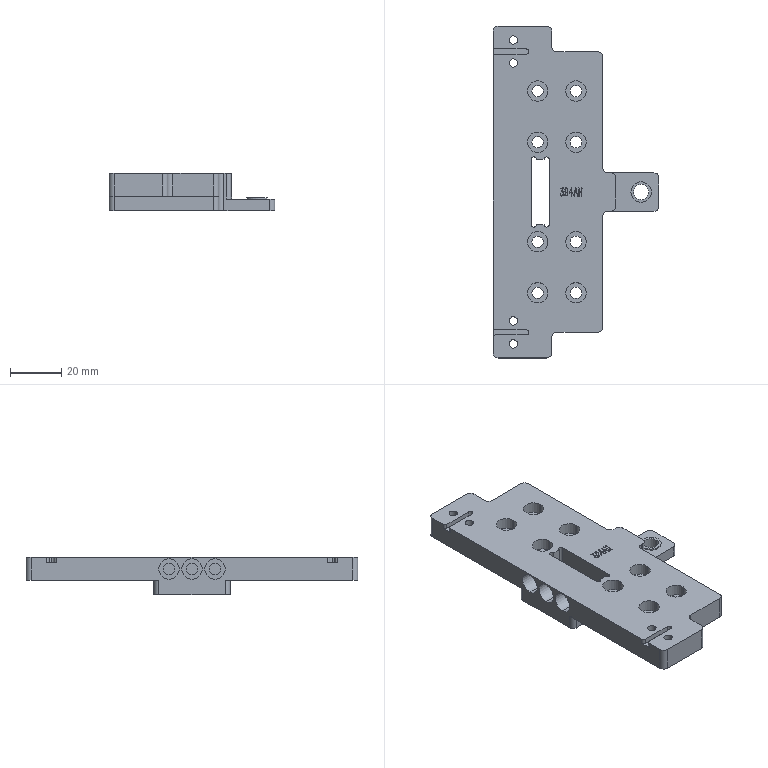NC program | NX | posted with a generic post | part box 65 x 130 x 14.5 mm
Lines 4087 to 4982 of 11202:
(ZLEVEL_PROFILE_COPY_COPY , TOOL : D3)
N8088 T16 M6
N8090 G54
N8092 G17 G0 G90 X9.873 Y-15.4 B0. C0. S9500 M3
N8094 G43 Z30. H16
N8096 Z-0.199
N8098 G94 G1 X10.133 Y-15.85 F1000.
N8100 G3 X10.393 Y-16. R0.3
N8102 G1 X11.336 F1200.
N8104 G2 X11.25 Y-15.5 R1.5
N8106 G1 Y-15.124
N8108 G3 X11.1 Y-14.864 R0.3
N8110 G1 X10.65 Y-14.604
N8112 G0 X9.873 Y-15.4 Z-0.397
N8114 G1 X10.133 Y-15.85 F1000.
N8116 G3 X10.393 Y-16. R0.3
N8118 G1 X11.336 F1200.
N8120 G2 X11.25 Y-15.5 R1.5
N8122 G1 Y-15.124
N8124 G3 X11.1 Y-14.864 R0.3
N8126 G1 X10.65 Y-14.604
N8128 G0 X9.873 Y-15.4 Z-0.596
N8130 G1 X10.133 Y-15.85 F1000.
N8132 G3 X10.393 Y-16. R0.3
N8134 G1 X11.336 F1200.
N8136 G2 X11.25 Y-15.5 R1.5
N8138 G1 Y-15.124
N8140 G3 X11.1 Y-14.864 R0.3
N8142 G1 X10.65 Y-14.604
N8144 G0 X9.873 Y-15.4 Z-0.795
N8146 G1 X10.133 Y-15.85 F1000.
N8148 G3 X10.393 Y-16. R0.3
N8150 G1 X11.336 F1200.
N8152 G2 X11.25 Y-15.5 R1.5
N8154 G1 Y-15.124
N8156 G3 X11.1 Y-14.864 R0.3
N8158 G1 X10.65 Y-14.604
N8160 G0 X9.873 Y-15.4 Z-0.993
N8162 G1 X10.133 Y-15.85 F1000.
N8164 G3 X10.393 Y-16. R0.3
N8166 G1 X11.336 F1200.
N8168 G2 X11.25 Y-15.5 R1.5
N8170 G1 Y-15.124
N8172 G3 X11.1 Y-14.864 R0.3
N8174 G1 X10.65 Y-14.604
N8176 G0 X9.873 Y-15.4 Z-1.192
N8178 G1 X10.133 Y-15.85 F1000.
N8180 G3 X10.393 Y-16. R0.3
N8182 G1 X11.336 F1200.
N8184 G2 X11.25 Y-15.5 R1.5
N8186 G1 Y-15.124
N8188 G3 X11.1 Y-14.864 R0.3
N8190 G1 X10.65 Y-14.604
N8192 G0 X9.873 Y-15.4 Z-1.39
N8194 G1 X10.133 Y-15.85 F1000.
N8196 G3 X10.393 Y-16. R0.3
N8198 G1 X11.336 F1200.
N8200 G2 X11.25 Y-15.5 R1.5
N8202 G1 Y-15.124
N8204 G3 X11.1 Y-14.864 R0.3
N8206 G1 X10.65 Y-14.604
N8208 G0 X9.873 Y-15.4 Z-1.589
N8210 G1 X10.133 Y-15.85 F1000.
N8212 G3 X10.393 Y-16. R0.3
N8214 G1 X11.336 F1200.
N8216 G2 X11.25 Y-15.5 R1.5
N8218 G1 Y-15.124
N8220 G3 X11.1 Y-14.864 R0.3
N8222 G1 X10.65 Y-14.604
N8224 G0 X9.873 Y-15.4 Z-1.788
N8226 G1 X10.133 Y-15.85 F1000.
N8228 G3 X10.393 Y-16. R0.3
N8230 G1 X11.336 F1200.
N8232 G2 X11.25 Y-15.5 R1.5
N8234 G1 Y-15.124
N8236 G3 X11.1 Y-14.864 R0.3
N8238 G1 X10.65 Y-14.604
N8240 G0 X9.873 Y-15.4 Z-1.986
N8242 G1 X10.133 Y-15.85 F1000.
N8244 G3 X10.393 Y-16. R0.3
N8246 G1 X11.336 F1200.
N8248 G2 X11.25 Y-15.5 R1.5
N8250 G1 Y-15.124
N8252 G3 X11.1 Y-14.864 R0.3
N8254 G1 X10.65 Y-14.604
N8256 G0 X9.873 Y-15.4 Z-2.185
N8258 G1 X10.133 Y-15.85 F1000.
N8260 G3 X10.393 Y-16. R0.3
N8262 G1 X11.336 F1200.
N8264 G2 X11.25 Y-15.5 R1.5
N8266 G1 Y-15.124
N8268 G3 X11.1 Y-14.864 R0.3
N8270 G1 X10.65 Y-14.604
N8272 G0 X9.873 Y-15.4 Z-2.384
N8274 G1 X10.133 Y-15.85 F1000.
N8276 G3 X10.393 Y-16. R0.3
N8278 G1 X11.336 F1200.
N8280 G2 X11.25 Y-15.5 R1.5
N8282 G1 Y-15.124
N8284 G3 X11.1 Y-14.864 R0.3
N8286 G1 X10.65 Y-14.604
N8288 G0 X9.873 Y-15.4 Z-2.582
N8290 G1 X10.133 Y-15.85 F1000.
N8292 G3 X10.393 Y-16. R0.3
N8294 G1 X11.336 F1200.
N8296 G2 X11.25 Y-15.5 R1.5
N8298 G1 Y-15.124
N8300 G3 X11.1 Y-14.864 R0.3
N8302 G1 X10.65 Y-14.604
N8304 G0 X9.873 Y-15.4 Z-2.781
N8306 G1 X10.133 Y-15.85 F1000.
N8308 G3 X10.393 Y-16. R0.3
N8310 G1 X11.336 F1200.
N8312 G2 X11.25 Y-15.5 R1.5
N8314 G1 Y-15.124
N8316 G3 X11.1 Y-14.864 R0.3
N8318 G1 X10.65 Y-14.604
N8320 G0 X9.873 Y-15.4 Z-2.979
N8322 G1 X10.133 Y-15.85 F1000.
N8324 G3 X10.393 Y-16. R0.3
N8326 G1 X11.336 F1200.
N8328 G2 X11.25 Y-15.5 R1.5
N8330 G1 Y-15.124
N8332 G3 X11.1 Y-14.864 R0.3
N8334 G1 X10.65 Y-14.604
N8336 G0 X9.873 Y-15.4 Z-3.178
N8338 G1 X10.133 Y-15.85 F1000.
N8340 G3 X10.393 Y-16. R0.3
N8342 G1 X11.336 F1200.
N8344 G2 X11.25 Y-15.5 R1.5
N8346 G1 Y-15.124
N8348 G3 X11.1 Y-14.864 R0.3
N8350 G1 X10.65 Y-14.604
N8352 G0 X9.873 Y-15.4 Z-3.377
N8354 G1 X10.133 Y-15.85 F1000.
N8356 G3 X10.393 Y-16. R0.3
N8358 G1 X11.336 F1200.
N8360 G2 X11.25 Y-15.5 R1.5
N8362 G1 Y-15.124
N8364 G3 X11.1 Y-14.864 R0.3
N8366 G1 X10.65 Y-14.604
N8368 G0 X9.873 Y-15.4 Z-3.575
N8370 G1 X10.133 Y-15.85 F1000.
N8372 G3 X10.393 Y-16. R0.3
N8374 G1 X11.336 F1200.
N8376 G2 X11.25 Y-15.5 R1.5
N8378 G1 Y-15.124
N8380 G3 X11.1 Y-14.864 R0.3
N8382 G1 X10.65 Y-14.604
N8384 G0 X9.873 Y-15.4 Z-3.774
N8386 G1 X10.133 Y-15.85 F1000.
N8388 G3 X10.393 Y-16. R0.3
N8390 G1 X11.336 F1200.
N8392 G2 X11.25 Y-15.5 R1.5
N8394 G1 Y-15.124
N8396 G3 X11.1 Y-14.864 R0.3
N8398 G1 X10.65 Y-14.604
N8400 G0 X9.873 Y-15.4 Z-3.973
N8402 G1 X10.133 Y-15.85 F1000.
N8404 G3 X10.393 Y-16. R0.3
N8406 G1 X11.336 F1200.
N8408 G2 X11.25 Y-15.5 R1.5
N8410 G1 Y-15.124
N8412 G3 X11.1 Y-14.864 R0.3
N8414 G1 X10.65 Y-14.604
N8416 G0 X9.873 Y-15.4 Z-4.171
N8418 G1 X10.133 Y-15.85 F1000.
N8420 G3 X10.393 Y-16. R0.3
N8422 G1 X11.336 F1200.
N8424 G2 X11.25 Y-15.5 R1.5
N8426 G1 Y-15.124
N8428 G3 X11.1 Y-14.864 R0.3
N8430 G1 X10.65 Y-14.604
N8432 G0 X9.873 Y-15.4 Z-4.37
N8434 G1 X10.133 Y-15.85 F1000.
N8436 G3 X10.393 Y-16. R0.3
N8438 G1 X11.336 F1200.
N8440 G2 X11.25 Y-15.5 R1.5
N8442 G1 Y-15.124
N8444 G3 X11.1 Y-14.864 R0.3
N8446 G1 X10.65 Y-14.604
N8448 G0 X9.873 Y-15.4 Z-4.568
N8450 G1 X10.133 Y-15.85 F1000.
N8452 G3 X10.393 Y-16. R0.3
N8454 G1 X11.336 F1200.
N8456 G2 X11.25 Y-15.5 R1.5
N8458 G1 Y-15.124
N8460 G3 X11.1 Y-14.864 R0.3
N8462 G1 X10.65 Y-14.604
N8464 G0 X9.873 Y-15.4 Z-4.767
N8466 G1 X10.133 Y-15.85 F1000.
N8468 G3 X10.393 Y-16. R0.3
N8470 G1 X11.336 F1200.
N8472 G2 X11.25 Y-15.5 R1.5
N8474 G1 Y-15.124
N8476 G3 X11.1 Y-14.864 R0.3
N8478 G1 X10.65 Y-14.604
N8480 G0 X9.873 Y-15.4 Z-4.966
N8482 G1 X10.133 Y-15.85 F1000.
N8484 G3 X10.393 Y-16. R0.3
N8486 G1 X11.336 F1200.
N8488 G2 X11.25 Y-15.5 R1.5
N8490 G1 Y-15.124
N8492 G3 X11.1 Y-14.864 R0.3
N8494 G1 X10.65 Y-14.604
N8496 G0 X9.873 Y-15.4 Z-5.164
N8498 G1 X10.133 Y-15.85 F1000.
N8500 G3 X10.393 Y-16. R0.3
N8502 G1 X11.336 F1200.
N8504 G2 X11.25 Y-15.5 R1.5
N8506 G1 Y-15.124
N8508 G3 X11.1 Y-14.864 R0.3
N8510 G1 X10.65 Y-14.604
N8512 G0 X9.873 Y-15.4 Z-5.363
N8514 G1 X10.133 Y-15.85 F1000.
N8516 G3 X10.393 Y-16. R0.3
N8518 G1 X11.336 F1200.
N8520 G2 X11.25 Y-15.5 R1.5
N8522 G1 Y-15.124
N8524 G3 X11.1 Y-14.864 R0.3
N8526 G1 X10.65 Y-14.604
N8528 G0 X9.873 Y-15.4 Z-5.562
N8530 G1 X10.133 Y-15.85 F1000.
N8532 G3 X10.393 Y-16. R0.3
N8534 G1 X11.336 F1200.
N8536 G2 X11.25 Y-15.5 R1.5
N8538 G1 Y-15.124
N8540 G3 X11.1 Y-14.864 R0.3
N8542 G1 X10.65 Y-14.604
N8544 G0 X9.873 Y-15.4 Z-5.76
N8546 G1 X10.133 Y-15.85 F1000.
N8548 G3 X10.393 Y-16. R0.3
N8550 G1 X11.336 F1200.
N8552 G2 X11.25 Y-15.5 R1.5
N8554 G1 Y-15.124
N8556 G3 X11.1 Y-14.864 R0.3
N8558 G1 X10.65 Y-14.604
N8560 G0 X9.873 Y-15.4 Z-5.959
N8562 G1 X10.133 Y-15.85 F1000.
N8564 G3 X10.393 Y-16. R0.3
N8566 G1 X11.336 F1200.
N8568 G2 X11.25 Y-15.5 R1.5
N8570 G1 Y-15.124
N8572 G3 X11.1 Y-14.864 R0.3
N8574 G1 X10.65 Y-14.604
N8576 G0 X9.873 Y-15.4 Z-6.158
N8578 G1 X10.133 Y-15.85 F1000.
N8580 G3 X10.393 Y-16. R0.3
N8582 G1 X11.336 F1200.
N8584 G2 X11.25 Y-15.5 R1.5
N8586 G1 Y-15.124
N8588 G3 X11.1 Y-14.864 R0.3
N8590 G1 X10.65 Y-14.604
N8592 G0 X9.873 Y-15.4 Z-6.356
N8594 G1 X10.133 Y-15.85 F1000.
N8596 G3 X10.393 Y-16. R0.3
N8598 G1 X11.336 F1200.
N8600 G2 X11.25 Y-15.5 R1.5
N8602 G1 Y-15.124
N8604 G3 X11.1 Y-14.864 R0.3
N8606 G1 X10.65 Y-14.604
N8608 G0 X9.873 Y-15.4 Z-6.555
N8610 G1 X10.133 Y-15.85 F1000.
N8612 G3 X10.393 Y-16. R0.3
N8614 G1 X11.336 F1200.
N8616 G2 X11.25 Y-15.5 R1.5
N8618 G1 Y-15.124
N8620 G3 X11.1 Y-14.864 R0.3
N8622 G1 X10.65 Y-14.604
N8624 G0 X9.873 Y-15.4 Z-6.753
N8626 G1 X10.133 Y-15.85 F1000.
N8628 G3 X10.393 Y-16. R0.3
N8630 G1 X11.336 F1200.
N8632 G2 X11.25 Y-15.5 R1.5
N8634 G1 Y-15.124
N8636 G3 X11.1 Y-14.864 R0.3
N8638 G1 X10.65 Y-14.604
N8640 G0 X9.873 Y-15.4 Z-6.952
N8642 G1 X10.133 Y-15.85 F1000.
N8644 G3 X10.393 Y-16. R0.3
N8646 G1 X11.336 F1200.
N8648 G2 X11.25 Y-15.5 R1.5
N8650 G1 Y-15.124
N8652 G3 X11.1 Y-14.864 R0.3
N8654 G1 X10.65 Y-14.604
N8656 G0 X9.873 Y-15.4 Z-7.151
N8658 G1 X10.133 Y-15.85 F1000.
N8660 G3 X10.393 Y-16. R0.3
N8662 G1 X11.336 F1200.
N8664 G2 X11.25 Y-15.5 R1.5
N8666 G1 Y-15.124
N8668 G3 X11.1 Y-14.864 R0.3
N8670 G1 X10.65 Y-14.604
N8672 G0 X9.873 Y-15.4 Z-7.349
N8674 G1 X10.133 Y-15.85 F1000.
N8676 G3 X10.393 Y-16. R0.3
N8678 G1 X11.336 F1200.
N8680 G2 X11.25 Y-15.5 R1.5
N8682 G1 Y-15.124
N8684 G3 X11.1 Y-14.864 R0.3
N8686 G1 X10.65 Y-14.604
N8688 G0 X9.873 Y-15.4 Z-7.548
N8690 G1 X10.133 Y-15.85 F1000.
N8692 G3 X10.393 Y-16. R0.3
N8694 G1 X11.336 F1200.
N8696 G2 X11.25 Y-15.5 R1.5
N8698 G1 Y-15.124
N8700 G3 X11.1 Y-14.864 R0.3
N8702 G1 X10.65 Y-14.604
N8704 G0 X9.873 Y-15.4 Z-7.747
N8706 G1 X10.133 Y-15.85 F1000.
N8708 G3 X10.393 Y-16. R0.3
N8710 G1 X11.336 F1200.
N8712 G2 X11.25 Y-15.5 R1.5
N8714 G1 Y-15.124
N8716 G3 X11.1 Y-14.864 R0.3
N8718 G1 X10.65 Y-14.604
N8720 G0 X9.873 Y-15.4 Z-7.945
N8722 G1 X10.133 Y-15.85 F1000.
N8724 G3 X10.393 Y-16. R0.3
N8726 G1 X11.336 F1200.
N8728 G2 X11.25 Y-15.5 R1.5
N8730 G1 Y-15.124
N8732 G3 X11.1 Y-14.864 R0.3
N8734 G1 X10.65 Y-14.604
N8736 G0 X9.873 Y-15.4 Z-8.144
N8738 G1 X10.133 Y-15.85 F1000.
N8740 G3 X10.393 Y-16. R0.3
N8742 G1 X11.336 F1200.
N8744 G2 X11.25 Y-15.5 R1.5
N8746 G1 Y-15.124
N8748 G3 X11.1 Y-14.864 R0.3
N8750 G1 X10.65 Y-14.604
N8752 G0 X9.873 Y-15.4 Z-8.342
N8754 G1 X10.133 Y-15.85 F1000.
N8756 G3 X10.393 Y-16. R0.3
N8758 G1 X11.336 F1200.
N8760 G2 X11.25 Y-15.5 R1.5
N8762 G1 Y-15.124
N8764 G3 X11.1 Y-14.864 R0.3
N8766 G1 X10.65 Y-14.604
N8768 G0 X9.873 Y-15.4 Z-8.541
N8770 G1 X10.133 Y-15.85 F1000.
N8772 G3 X10.393 Y-16. R0.3
N8774 G1 X11.336 F1200.
N8776 G2 X11.25 Y-15.5 R1.5
N8778 G1 Y-15.124
N8780 G3 X11.1 Y-14.864 R0.3
N8782 G1 X10.65 Y-14.604
N8784 G0 X9.873 Y-15.4 Z-8.74
N8786 G1 X10.133 Y-15.85 F1000.
N8788 G3 X10.393 Y-16. R0.3
N8790 G1 X11.336 F1200.
N8792 G2 X11.25 Y-15.5 R1.5
N8794 G1 Y-15.124
N8796 G3 X11.1 Y-14.864 R0.3
N8798 G1 X10.65 Y-14.604
N8800 G0 X9.873 Y-15.4 Z-8.938
N8802 G1 X10.133 Y-15.85 F1000.
N8804 G3 X10.393 Y-16. R0.3
N8806 G1 X11.336 F1200.
N8808 G2 X11.25 Y-15.5 R1.5
N8810 G1 Y-15.124
N8812 G3 X11.1 Y-14.864 R0.3
N8814 G1 X10.65 Y-14.604
N8816 G0 X9.873 Y-15.4 Z-9.137
N8818 G1 X10.133 Y-15.85 F1000.
N8820 G3 X10.393 Y-16. R0.3
N8822 G1 X11.336 F1200.
N8824 G2 X11.25 Y-15.5 R1.5
N8826 G1 Y-15.124
N8828 G3 X11.1 Y-14.864 R0.3
N8830 G1 X10.65 Y-14.604
N8832 G0 X9.873 Y-15.4 Z-9.336
N8834 G1 X10.133 Y-15.85 F1000.
N8836 G3 X10.393 Y-16. R0.3
N8838 G1 X11.336 F1200.
N8840 G2 X11.25 Y-15.5 R1.5
N8842 G1 Y-15.124
N8844 G3 X11.1 Y-14.864 R0.3
N8846 G1 X10.65 Y-14.604
N8848 G0 X9.873 Y-15.4 Z-9.534
N8850 G1 X10.133 Y-15.85 F1000.
N8852 G3 X10.393 Y-16. R0.3
N8854 G1 X11.336 F1200.
N8856 G2 X11.25 Y-15.5 R1.5
N8858 G1 Y-15.124
N8860 G3 X11.1 Y-14.864 R0.3
N8862 G1 X10.65 Y-14.604
N8864 G0 X9.873 Y-15.4 Z-9.733
N8866 G1 X10.133 Y-15.85 F1000.
N8868 G3 X10.393 Y-16. R0.3
N8870 G1 X11.336 F1200.
N8872 G2 X11.25 Y-15.5 R1.5
N8874 G1 Y-15.124
N8876 G3 X11.1 Y-14.864 R0.3
N8878 G1 X10.65 Y-14.604
N8880 G0 X9.873 Y-15.4 Z-9.932
N8882 G1 X10.133 Y-15.85 F1000.
N8884 G3 X10.393 Y-16. R0.3
N8886 G1 X11.336 F1200.
N8888 G2 X11.25 Y-15.5 R1.5
N8890 G1 Y-15.124
N8892 G3 X11.1 Y-14.864 R0.3
N8894 G1 X10.65 Y-14.604
N8896 G0 X9.873 Y-15.4 Z-10.13
N8898 G1 X10.133 Y-15.85 F1000.
N8900 G3 X10.393 Y-16. R0.3
N8902 G1 X11.336 F1200.
N8904 G2 X11.25 Y-15.5 R1.5
N8906 G1 Y-15.124
N8908 G3 X11.1 Y-14.864 R0.3
N8910 G1 X10.65 Y-14.604
N8912 G0 X9.873 Y-15.4 Z-10.329
N8914 G1 X10.133 Y-15.85 F1000.
N8916 G3 X10.393 Y-16. R0.3
N8918 G1 X11.336 F1200.
N8920 G2 X11.25 Y-15.5 R1.5
N8922 G1 Y-15.124
N8924 G3 X11.1 Y-14.864 R0.3
N8926 G1 X10.65 Y-14.604
N8928 G0 X9.873 Y-15.4 Z-10.527
N8930 G1 X10.133 Y-15.85 F1000.
N8932 G3 X10.393 Y-16. R0.3
N8934 G1 X11.336 F1200.
N8936 G2 X11.25 Y-15.5 R1.5
N8938 G1 Y-15.124
N8940 G3 X11.1 Y-14.864 R0.3
N8942 G1 X10.65 Y-14.604
N8944 G0 X9.873 Y-15.4 Z-10.726
N8946 G1 X10.133 Y-15.85 F1000.
N8948 G3 X10.393 Y-16. R0.3
N8950 G1 X11.336 F1200.
N8952 G2 X11.25 Y-15.5 R1.5
N8954 G1 Y-15.124
N8956 G3 X11.1 Y-14.864 R0.3
N8958 G1 X10.65 Y-14.604
N8960 G0 X9.873 Y-15.4 Z-10.925
N8962 G1 X10.133 Y-15.85 F1000.
N8964 G3 X10.393 Y-16. R0.3
N8966 G1 X11.336 F1200.
N8968 G2 X11.25 Y-15.5 R1.5
N8970 G1 Y-15.124
N8972 G3 X11.1 Y-14.864 R0.3
N8974 G1 X10.65 Y-14.604
N8976 G0 X9.873 Y-15.4 Z-11.123
N8978 G1 X10.133 Y-15.85 F1000.
N8980 G3 X10.393 Y-16. R0.3
N8982 G1 X11.336 F1200.
N8984 G2 X11.25 Y-15.5 R1.5
N8986 G1 Y-15.124
N8988 G3 X11.1 Y-14.864 R0.3
N8990 G1 X10.65 Y-14.604
N8992 G0 X9.873 Y-15.4 Z-11.322
N8994 G1 X10.133 Y-15.85 F1000.
N8996 G3 X10.393 Y-16. R0.3
N8998 G1 X11.336 F1200.
N9000 G2 X11.25 Y-15.5 R1.5
N9002 G1 Y-15.124
N9004 G3 X11.1 Y-14.864 R0.3
N9006 G1 X10.65 Y-14.604
N9008 G0 X9.873 Y-15.4 Z-11.521
N9010 G1 X10.133 Y-15.85 F1000.
N9012 G3 X10.393 Y-16. R0.3
N9014 G1 X11.336 F1200.
N9016 G2 X11.25 Y-15.5 R1.5
N9018 G1 Y-15.124
N9020 G3 X11.1 Y-14.864 R0.3
N9022 G1 X10.65 Y-14.604
N9024 G0 X9.873 Y-15.4 Z-11.719
N9026 G1 X10.133 Y-15.85 F1000.
N9028 G3 X10.393 Y-16. R0.3
N9030 G1 X11.336 F1200.
N9032 G2 X11.25 Y-15.5 R1.5
N9034 G1 Y-15.124
N9036 G3 X11.1 Y-14.864 R0.3
N9038 G1 X10.65 Y-14.604
N9040 G0 X9.873 Y-15.4 Z-11.918
N9042 G1 X10.133 Y-15.85 F1000.
N9044 G3 X10.393 Y-16. R0.3
N9046 G1 X11.336 F1200.
N9048 G2 X11.25 Y-15.5 R1.5
N9050 G1 Y-15.124
N9052 G3 X11.1 Y-14.864 R0.3
N9054 G1 X10.65 Y-14.604
N9056 G0 X9.873 Y-15.4 Z-12.116
N9058 G1 X10.133 Y-15.85 F1000.
N9060 G3 X10.393 Y-16. R0.3
N9062 G1 X11.336 F1200.
N9064 G2 X11.25 Y-15.5 R1.5
N9066 G1 Y-15.124
N9068 G3 X11.1 Y-14.864 R0.3
N9070 G1 X10.65 Y-14.604
N9072 G0 X9.873 Y-15.4 Z-12.315
N9074 G1 X10.133 Y-15.85 F1000.
N9076 G3 X10.393 Y-16. R0.3
N9078 G1 X11.336 F1200.
N9080 G2 X11.25 Y-15.5 R1.5
N9082 G1 Y-15.124
N9084 G3 X11.1 Y-14.864 R0.3
N9086 G1 X10.65 Y-14.604
N9088 G0 X9.873 Y-15.4 Z-12.514
N9090 G1 X10.133 Y-15.85 F1000.
N9092 G3 X10.393 Y-16. R0.3
N9094 G1 X11.336 F1200.
N9096 G2 X11.25 Y-15.5 R1.5
N9098 G1 Y-15.124
N9100 G3 X11.1 Y-14.864 R0.3
N9102 G1 X10.65 Y-14.604
N9104 G0 X9.873 Y-15.4 Z-12.712
N9106 G1 X10.133 Y-15.85 F1000.
N9108 G3 X10.393 Y-16. R0.3
N9110 G1 X11.336 F1200.
N9112 G2 X11.25 Y-15.5 R1.5
N9114 G1 Y-15.124
N9116 G3 X11.1 Y-14.864 R0.3
N9118 G1 X10.65 Y-14.604
N9120 G0 X9.873 Y-15.4 Z-12.911
N9122 G1 X10.133 Y-15.85 F1000.
N9124 G3 X10.393 Y-16. R0.3
N9126 G1 X11.336 F1200.
N9128 G2 X11.25 Y-15.5 R1.5
N9130 G1 Y-15.124
N9132 G3 X11.1 Y-14.864 R0.3
N9134 G1 X10.65 Y-14.604
N9136 G0 X9.873 Y-15.4 Z-13.11
N9138 G1 X10.133 Y-15.85 F1000.
N9140 G3 X10.393 Y-16. R0.3
N9142 G1 X11.336 F1200.
N9144 G2 X11.25 Y-15.5 R1.5
N9146 G1 Y-15.124
N9148 G3 X11.1 Y-14.864 R0.3
N9150 G1 X10.65 Y-14.604
N9152 G0 X9.873 Y-15.4 Z-13.308
N9154 G1 X10.133 Y-15.85 F1000.
N9156 G3 X10.393 Y-16. R0.3
N9158 G1 X11.336 F1200.
N9160 G2 X11.25 Y-15.5 R1.5
N9162 G1 Y-15.124
N9164 G3 X11.1 Y-14.864 R0.3
N9166 G1 X10.65 Y-14.604
N9168 G0 X9.873 Y-15.4 Z-13.507
N9170 G1 X10.133 Y-15.85 F1000.
N9172 G3 X10.393 Y-16. R0.3
N9174 G1 X11.336 F1200.
N9176 G2 X11.25 Y-15.5 R1.5
N9178 G1 Y-15.124
N9180 G3 X11.1 Y-14.864 R0.3
N9182 G1 X10.65 Y-14.604
N9184 G0 X9.873 Y-15.4 Z-13.705
N9186 G1 X10.133 Y-15.85 F1000.
N9188 G3 X10.393 Y-16. R0.3
N9190 G1 X11.336 F1200.
N9192 G2 X11.25 Y-15.5 R1.5
N9194 G1 Y-15.124
N9196 G3 X11.1 Y-14.864 R0.3
N9198 G1 X10.65 Y-14.604
N9200 G0 X9.873 Y-15.4 Z-13.904
N9202 G1 X10.133 Y-15.85 F1000.
N9204 G3 X10.393 Y-16. R0.3
N9206 G1 X11.336 F1200.
N9208 G2 X11.25 Y-15.5 R1.5
N9210 G1 Y-15.124
N9212 G3 X11.1 Y-14.864 R0.3
N9214 G1 X10.65 Y-14.604
N9216 G0 X9.873 Y-15.4 Z-14.103
N9218 G1 X10.133 Y-15.85 F1000.
N9220 G3 X10.393 Y-16. R0.3
N9222 G1 X11.336 F1200.
N9224 G2 X11.25 Y-15.5 R1.5
N9226 G1 Y-15.124
N9228 G3 X11.1 Y-14.864 R0.3
N9230 G1 X10.65 Y-14.604
N9232 G0 X9.873 Y-15.4 Z-14.301
N9234 G1 X10.133 Y-15.85 F1000.
N9236 G3 X10.393 Y-16. R0.3
N9238 G1 X11.336 F1200.
N9240 G2 X11.25 Y-15.5 R1.5
N9242 G1 Y-15.124
N9244 G3 X11.1 Y-14.864 R0.3
N9246 G1 X10.65 Y-14.604
N9248 G0 X9.873 Y-15.4 Z-14.5
N9250 G1 X10.133 Y-15.85 F1000.
N9252 G3 X10.393 Y-16. R0.3
N9254 G1 X11.336 F1200.
N9256 G2 X11.25 Y-15.5 R1.5
N9258 G1 Y-15.124
N9260 G3 X11.1 Y-14.864 R0.3
N9262 G1 X10.65 Y-14.604
N9264 G0 Z30.
N9266 Y-13.396
N9268 Z-0.199
N9270 G1 X11.1 Y-13.136 F1000.
N9272 G3 X11.25 Y-12.876 R0.3
N9274 G1 Y-12.5 F1200.
N9276 G2 X11.336 Y-12. R1.5
N9278 G1 X10.393
N9280 G3 X10.133 Y-12.15 R0.3
N9282 G1 X9.873 Y-12.6
N9284 G0 X10.65 Y-13.396 Z-0.397
N9286 G1 X11.1 Y-13.136 F1000.
N9288 G3 X11.25 Y-12.876 R0.3
N9290 G1 Y-12.5 F1200.
N9292 G2 X11.336 Y-12. R1.5
N9294 G1 X10.393
N9296 G3 X10.133 Y-12.15 R0.3
N9298 G1 X9.873 Y-12.6
N9300 G0 X10.65 Y-13.396 Z-0.596
N9302 G1 X11.1 Y-13.136 F1000.
N9304 G3 X11.25 Y-12.876 R0.3
N9306 G1 Y-12.5 F1200.
N9308 G2 X11.336 Y-12. R1.5
N9310 G1 X10.393
N9312 G3 X10.133 Y-12.15 R0.3
N9314 G1 X9.873 Y-12.6
N9316 G0 X10.65 Y-13.396 Z-0.795
N9318 G1 X11.1 Y-13.136 F1000.
N9320 G3 X11.25 Y-12.876 R0.3
N9322 G1 Y-12.5 F1200.
N9324 G2 X11.336 Y-12. R1.5
N9326 G1 X10.393
N9328 G3 X10.133 Y-12.15 R0.3
N9330 G1 X9.873 Y-12.6
N9332 G0 X10.65 Y-13.396 Z-0.993
N9334 G1 X11.1 Y-13.136 F1000.
N9336 G3 X11.25 Y-12.876 R0.3
N9338 G1 Y-12.5 F1200.
N9340 G2 X11.336 Y-12. R1.5
N9342 G1 X10.393
N9344 G3 X10.133 Y-12.15 R0.3
N9346 G1 X9.873 Y-12.6
N9348 G0 X10.65 Y-13.396 Z-1.192
N9350 G1 X11.1 Y-13.136 F1000.
N9352 G3 X11.25 Y-12.876 R0.3
N9354 G1 Y-12.5 F1200.
N9356 G2 X11.336 Y-12. R1.5
N9358 G1 X10.393
N9360 G3 X10.133 Y-12.15 R0.3
N9362 G1 X9.873 Y-12.6
N9364 G0 X10.65 Y-13.396 Z-1.39
N9366 G1 X11.1 Y-13.136 F1000.
N9368 G3 X11.25 Y-12.876 R0.3
N9370 G1 Y-12.5 F1200.
N9372 G2 X11.336 Y-12. R1.5
N9374 G1 X10.393
N9376 G3 X10.133 Y-12.15 R0.3
N9378 G1 X9.873 Y-12.6
N9380 G0 X10.65 Y-13.396 Z-1.589
N9382 G1 X11.1 Y-13.136 F1000.
N9384 G3 X11.25 Y-12.876 R0.3
N9386 G1 Y-12.5 F1200.
N9388 G2 X11.336 Y-12. R1.5
N9390 G1 X10.393
N9392 G3 X10.133 Y-12.15 R0.3
N9394 G1 X9.873 Y-12.6
N9396 G0 X10.65 Y-13.396 Z-1.788
N9398 G1 X11.1 Y-13.136 F1000.
N9400 G3 X11.25 Y-12.876 R0.3
N9402 G1 Y-12.5 F1200.
N9404 G2 X11.336 Y-12. R1.5
N9406 G1 X10.393
N9408 G3 X10.133 Y-12.15 R0.3
N9410 G1 X9.873 Y-12.6
N9412 G0 X10.65 Y-13.396 Z-1.986
N9414 G1 X11.1 Y-13.136 F1000.
N9416 G3 X11.25 Y-12.876 R0.3
N9418 G1 Y-12.5 F1200.
N9420 G2 X11.336 Y-12. R1.5
N9422 G1 X10.393
N9424 G3 X10.133 Y-12.15 R0.3
N9426 G1 X9.873 Y-12.6
N9428 G0 X10.65 Y-13.396 Z-2.185
N9430 G1 X11.1 Y-13.136 F1000.
N9432 G3 X11.25 Y-12.876 R0.3
N9434 G1 Y-12.5 F1200.
N9436 G2 X11.336 Y-12. R1.5
N9438 G1 X10.393
N9440 G3 X10.133 Y-12.15 R0.3
N9442 G1 X9.873 Y-12.6
N9444 G0 X10.65 Y-13.396 Z-2.384
N9446 G1 X11.1 Y-13.136 F1000.
N9448 G3 X11.25 Y-12.876 R0.3
N9450 G1 Y-12.5 F1200.
N9452 G2 X11.336 Y-12. R1.5
N9454 G1 X10.393
N9456 G3 X10.133 Y-12.15 R0.3
N9458 G1 X9.873 Y-12.6
N9460 G0 X10.65 Y-13.396 Z-2.582
N9462 G1 X11.1 Y-13.136 F1000.
N9464 G3 X11.25 Y-12.876 R0.3
N9466 G1 Y-12.5 F1200.
N9468 G2 X11.336 Y-12. R1.5
N9470 G1 X10.393
N9472 G3 X10.133 Y-12.15 R0.3
N9474 G1 X9.873 Y-12.6
N9476 G0 X10.65 Y-13.396 Z-2.781
N9478 G1 X11.1 Y-13.136 F1000.
N9480 G3 X11.25 Y-12.876 R0.3
N9482 G1 Y-12.5 F1200.
N9484 G2 X11.336 Y-12. R1.5
N9486 G1 X10.393
N9488 G3 X10.133 Y-12.15 R0.3
N9490 G1 X9.873 Y-12.6
N9492 G0 X10.65 Y-13.396 Z-2.979
N9494 G1 X11.1 Y-13.136 F1000.
N9496 G3 X11.25 Y-12.876 R0.3
N9498 G1 Y-12.5 F1200.
N9500 G2 X11.336 Y-12. R1.5
N9502 G1 X10.393
N9504 G3 X10.133 Y-12.15 R0.3
N9506 G1 X9.873 Y-12.6
N9508 G0 X10.65 Y-13.396 Z-3.178
N9510 G1 X11.1 Y-13.136 F1000.
N9512 G3 X11.25 Y-12.876 R0.3
N9514 G1 Y-12.5 F1200.
N9516 G2 X11.336 Y-12. R1.5
N9518 G1 X10.393
N9520 G3 X10.133 Y-12.15 R0.3
N9522 G1 X9.873 Y-12.6
N9524 G0 X10.65 Y-13.396 Z-3.377
N9526 G1 X11.1 Y-13.136 F1000.
N9528 G3 X11.25 Y-12.876 R0.3
N9530 G1 Y-12.5 F1200.
N9532 G2 X11.336 Y-12. R1.5
N9534 G1 X10.393
N9536 G3 X10.133 Y-12.15 R0.3
N9538 G1 X9.873 Y-12.6
N9540 G0 X10.65 Y-13.396 Z-3.575
N9542 G1 X11.1 Y-13.136 F1000.
N9544 G3 X11.25 Y-12.876 R0.3
N9546 G1 Y-12.5 F1200.
N9548 G2 X11.336 Y-12. R1.5
N9550 G1 X10.393
N9552 G3 X10.133 Y-12.15 R0.3
N9554 G1 X9.873 Y-12.6
N9556 G0 X10.65 Y-13.396 Z-3.774
N9558 G1 X11.1 Y-13.136 F1000.
N9560 G3 X11.25 Y-12.876 R0.3
N9562 G1 Y-12.5 F1200.
N9564 G2 X11.336 Y-12. R1.5
N9566 G1 X10.393
N9568 G3 X10.133 Y-12.15 R0.3
N9570 G1 X9.873 Y-12.6
N9572 G0 X10.65 Y-13.396 Z-3.973
N9574 G1 X11.1 Y-13.136 F1000.
N9576 G3 X11.25 Y-12.876 R0.3
N9578 G1 Y-12.5 F1200.
N9580 G2 X11.336 Y-12. R1.5
N9582 G1 X10.393
N9584 G3 X10.133 Y-12.15 R0.3
N9586 G1 X9.873 Y-12.6
N9588 G0 X10.65 Y-13.396 Z-4.171
N9590 G1 X11.1 Y-13.136 F1000.
N9592 G3 X11.25 Y-12.876 R0.3
N9594 G1 Y-12.5 F1200.
N9596 G2 X11.336 Y-12. R1.5
N9598 G1 X10.393
N9600 G3 X10.133 Y-12.15 R0.3
N9602 G1 X9.873 Y-12.6
N9604 G0 X10.65 Y-13.396 Z-4.37
N9606 G1 X11.1 Y-13.136 F1000.
N9608 G3 X11.25 Y-12.876 R0.3
N9610 G1 Y-12.5 F1200.
N9612 G2 X11.336 Y-12. R1.5
N9614 G1 X10.393
N9616 G3 X10.133 Y-12.15 R0.3
N9618 G1 X9.873 Y-12.6
N9620 G0 X10.65 Y-13.396 Z-4.568
N9622 G1 X11.1 Y-13.136 F1000.
N9624 G3 X11.25 Y-12.876 R0.3
N9626 G1 Y-12.5 F1200.
N9628 G2 X11.336 Y-12. R1.5
N9630 G1 X10.393
N9632 G3 X10.133 Y-12.15 R0.3
N9634 G1 X9.873 Y-12.6
N9636 G0 X10.65 Y-13.396 Z-4.767
N9638 G1 X11.1 Y-13.136 F1000.
N9640 G3 X11.25 Y-12.876 R0.3
N9642 G1 Y-12.5 F1200.
N9644 G2 X11.336 Y-12. R1.5
N9646 G1 X10.393
N9648 G3 X10.133 Y-12.15 R0.3
N9650 G1 X9.873 Y-12.6
N9652 G0 X10.65 Y-13.396 Z-4.966
N9654 G1 X11.1 Y-13.136 F1000.
N9656 G3 X11.25 Y-12.876 R0.3
N9658 G1 Y-12.5 F1200.
N9660 G2 X11.336 Y-12. R1.5
N9662 G1 X10.393
N9664 G3 X10.133 Y-12.15 R0.3
N9666 G1 X9.873 Y-12.6
N9668 G0 X10.65 Y-13.396 Z-5.164
N9670 G1 X11.1 Y-13.136 F1000.
N9672 G3 X11.25 Y-12.876 R0.3
N9674 G1 Y-12.5 F1200.
N9676 G2 X11.336 Y-12. R1.5
N9678 G1 X10.393
N9680 G3 X10.133 Y-12.15 R0.3
N9682 G1 X9.873 Y-12.6
N9684 G0 X10.65 Y-13.396 Z-5.363
N9686 G1 X11.1 Y-13.136 F1000.
N9688 G3 X11.25 Y-12.876 R0.3
N9690 G1 Y-12.5 F1200.
N9692 G2 X11.336 Y-12. R1.5
N9694 G1 X10.393
N9696 G3 X10.133 Y-12.15 R0.3
N9698 G1 X9.873 Y-12.6
N9700 G0 X10.65 Y-13.396 Z-5.562
N9702 G1 X11.1 Y-13.136 F1000.
N9704 G3 X11.25 Y-12.876 R0.3
N9706 G1 Y-12.5 F1200.
N9708 G2 X11.336 Y-12. R1.5
N9710 G1 X10.393
N9712 G3 X10.133 Y-12.15 R0.3
N9714 G1 X9.873 Y-12.6
N9716 G0 X10.65 Y-13.396 Z-5.76
N9718 G1 X11.1 Y-13.136 F1000.
N9720 G3 X11.25 Y-12.876 R0.3
N9722 G1 Y-12.5 F1200.
N9724 G2 X11.336 Y-12. R1.5
N9726 G1 X10.393
N9728 G3 X10.133 Y-12.15 R0.3
N9730 G1 X9.873 Y-12.6
N9732 G0 X10.65 Y-13.396 Z-5.959
N9734 G1 X11.1 Y-13.136 F1000.
N9736 G3 X11.25 Y-12.876 R0.3
N9738 G1 Y-12.5 F1200.
N9740 G2 X11.336 Y-12. R1.5
N9742 G1 X10.393
N9744 G3 X10.133 Y-12.15 R0.3
N9746 G1 X9.873 Y-12.6
N9748 G0 X10.65 Y-13.396 Z-6.158
N9750 G1 X11.1 Y-13.136 F1000.
N9752 G3 X11.25 Y-12.876 R0.3
N9754 G1 Y-12.5 F1200.
N9756 G2 X11.336 Y-12. R1.5
N9758 G1 X10.393
N9760 G3 X10.133 Y-12.15 R0.3
N9762 G1 X9.873 Y-12.6
N9764 G0 X10.65 Y-13.396 Z-6.356
N9766 G1 X11.1 Y-13.136 F1000.
N9768 G3 X11.25 Y-12.876 R0.3
N9770 G1 Y-12.5 F1200.
N9772 G2 X11.336 Y-12. R1.5
N9774 G1 X10.393
N9776 G3 X10.133 Y-12.15 R0.3
N9778 G1 X9.873 Y-12.6
N9780 G0 X10.65 Y-13.396 Z-6.555
N9782 G1 X11.1 Y-13.136 F1000.
N9784 G3 X11.25 Y-12.876 R0.3
N9786 G1 Y-12.5 F1200.
N9788 G2 X11.336 Y-12. R1.5
N9790 G1 X10.393
N9792 G3 X10.133 Y-12.15 R0.3
N9794 G1 X9.873 Y-12.6
N9796 G0 X10.65 Y-13.396 Z-6.753
N9798 G1 X11.1 Y-13.136 F1000.
N9800 G3 X11.25 Y-12.876 R0.3
N9802 G1 Y-12.5 F1200.
N9804 G2 X11.336 Y-12. R1.5
N9806 G1 X10.393
N9808 G3 X10.133 Y-12.15 R0.3
N9810 G1 X9.873 Y-12.6
N9812 G0 X10.65 Y-13.396 Z-6.952
N9814 G1 X11.1 Y-13.136 F1000.
N9816 G3 X11.25 Y-12.876 R0.3
N9818 G1 Y-12.5 F1200.
N9820 G2 X11.336 Y-12. R1.5
N9822 G1 X10.393
N9824 G3 X10.133 Y-12.15 R0.3
N9826 G1 X9.873 Y-12.6
N9828 G0 X10.65 Y-13.396 Z-7.151
N9830 G1 X11.1 Y-13.136 F1000.
N9832 G3 X11.25 Y-12.876 R0.3
N9834 G1 Y-12.5 F1200.
N9836 G2 X11.336 Y-12. R1.5
N9838 G1 X10.393
N9840 G3 X10.133 Y-12.15 R0.3
N9842 G1 X9.873 Y-12.6
N9844 G0 X10.65 Y-13.396 Z-7.349
N9846 G1 X11.1 Y-13.136 F1000.
N9848 G3 X11.25 Y-12.876 R0.3
N9850 G1 Y-12.5 F1200.
N9852 G2 X11.336 Y-12. R1.5
N9854 G1 X10.393
N9856 G3 X10.133 Y-12.15 R0.3
N9858 G1 X9.873 Y-12.6
N9860 G0 X10.65 Y-13.396 Z-7.548
N9862 G1 X11.1 Y-13.136 F1000.
N9864 G3 X11.25 Y-12.876 R0.3
N9866 G1 Y-12.5 F1200.
N9868 G2 X11.336 Y-12. R1.5
N9870 G1 X10.393
N9872 G3 X10.133 Y-12.15 R0.3